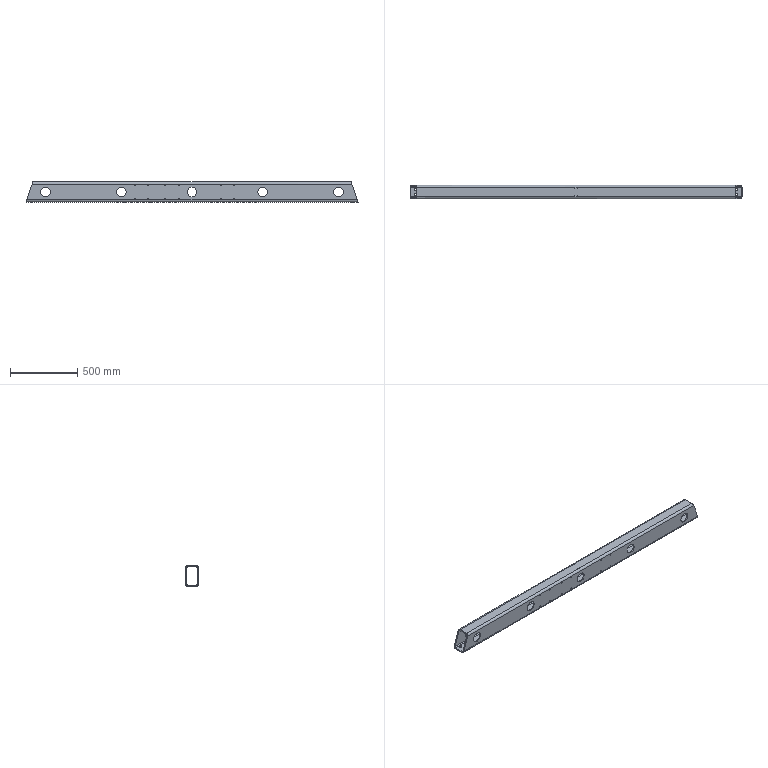Part | STEP file | 012-Rectangular tube 150x100x8_default<machining> | 1 solid | 78 faces | box 2470 x 100 x 150 mm | volume 8324006 mm3 | cylinder 68 | plane 10 | commonest cylinder face diameters 6.8 x24 72 x20 3.3 x8 18 x8 16 x4 32 x4